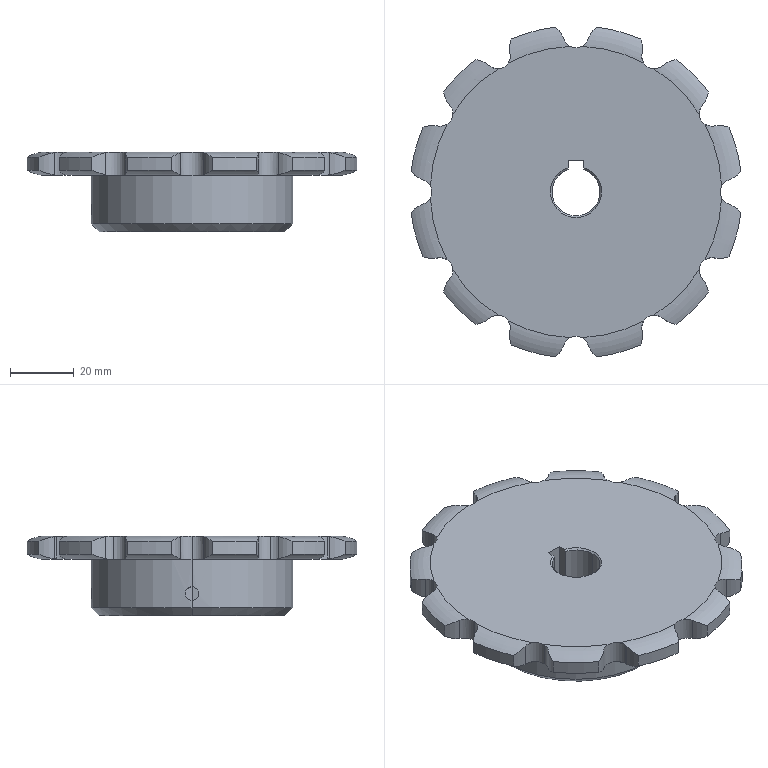Part | STEP file | 0228_104_Sprocket_RF2040S1200 | 1 solid | 102 faces | box 103.209 x 103.209 x 25 mm | volume 105106 mm3 | cylinder 64 | torus 24 | cone 8 | plane 6 | commonest cylinder face diameters 19.6 x26 7.92 x17 104 x12 4.2 x4 15 x3 63 x2